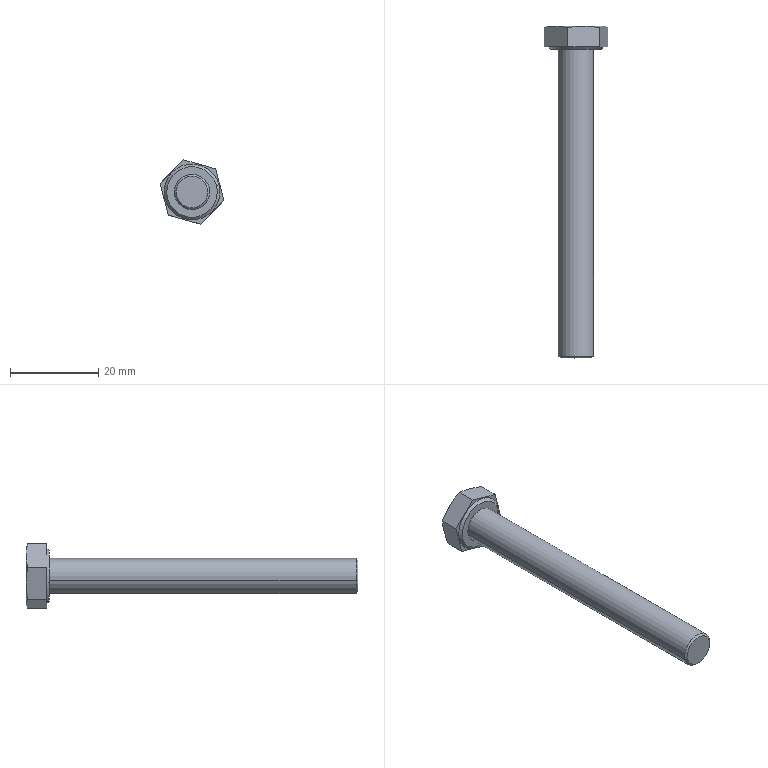Part | STEP file | 2026.6.15-Main Assembly图.sldasm-Part-12 | 1 solid | 22 faces | box 14.453 x 75.3 x 14.544 mm | volume 4272 mm3 | cone 10 | plane 10 | cylinder 2 | commonest cylinder face diameters 8 x2
STEP:
#1=CARTESIAN_POINT('',(-848.14,570.541,3100.088));
#2=VERTEX_POINT('',#1);
#3=CARTESIAN_POINT('',(-841.164,570.541,3101.869));
#4=VERTEX_POINT('',#3);
#5=CARTESIAN_POINT('',(-844.652,570.541,3100.979));
#6=DIRECTION('',(0.,-1.,0.));
#7=DIRECTION('',(-0.9689,0.,-0.2474));
#8=AXIS2_PLACEMENT_3D('',#5,#6,#7);
#9=CIRCLE('',#8,3.6);
#10=EDGE_CURVE('',#2,#4,#9,.T.);
#11=ORIENTED_EDGE('',*,*,#10,.F.);
#12=CARTESIAN_POINT('',(-848.527,570.941,3099.989));
#13=VERTEX_POINT('',#12);
#14=CARTESIAN_POINT('',(-848.14,570.541,3100.088));
#15=DIRECTION('',(-0.6851,0.7071,-0.1749));
#16=VECTOR('',#15,1000.);
#17=LINE('',#14,#16);
#18=EDGE_CURVE('',#2,#13,#17,.T.);
#19=ORIENTED_EDGE('',*,*,#18,.T.);
#20=CARTESIAN_POINT('',(-840.776,570.941,3101.968));
#21=VERTEX_POINT('',#20);
#22=CARTESIAN_POINT('',(-844.652,570.941,3100.979));
#23=DIRECTION('',(0.,1.,0.));
#24=DIRECTION('',(-0.9689,0.,-0.2474));
#25=AXIS2_PLACEMENT_3D('',#22,#23,#24);
#26=CIRCLE('',#25,4.);
#27=EDGE_CURVE('',#21,#13,#26,.T.);
#28=ORIENTED_EDGE('',*,*,#27,.F.);
#29=CARTESIAN_POINT('',(-841.164,570.541,3101.869));
#30=DIRECTION('',(0.6851,0.7071,0.1749));
#31=VECTOR('',#30,1000.);
#32=LINE('',#29,#31);
#33=EDGE_CURVE('',#4,#21,#32,.T.);
#34=ORIENTED_EDGE('',*,*,#33,.F.);
#35=EDGE_LOOP('',(#11,#19,#28,#34));
#36=FACE_OUTER_BOUND('',#35,.T.);
#37=CARTESIAN_POINT('',(-844.652,570.541,3100.979));
#38=DIRECTION('',(0.,1.,0.));
#39=DIRECTION('',(-0.9689,0.,-0.2474));
#40=AXIS2_PLACEMENT_3D('',#37,#38,#39);
#41=CONICAL_SURFACE('',#40,3.6,0.7854);
#42=ADVANCED_FACE('',(#36),#41,.T.);
#43=ORIENTED_EDGE('',*,*,#27,.T.);
#44=CARTESIAN_POINT('',(-848.527,640.541,3099.989));
#45=VERTEX_POINT('',#44);
#46=CARTESIAN_POINT('',(-848.527,570.541,3099.989));
#47=DIRECTION('',(0.,1.,0.));
#48=VECTOR('',#47,1000.);
#49=LINE('',#46,#48);
#50=EDGE_CURVE('',#13,#45,#49,.T.);
#51=ORIENTED_EDGE('',*,*,#50,.T.);
#52=CARTESIAN_POINT('',(-840.776,640.541,3101.968));
#53=VERTEX_POINT('',#52);
#54=CARTESIAN_POINT('',(-844.652,640.541,3100.979));
#55=DIRECTION('',(0.,-1.,0.));
#56=DIRECTION('',(0.9689,0.,0.2474));
#57=AXIS2_PLACEMENT_3D('',#54,#55,#56);
#58=CIRCLE('',#57,4.);
#59=EDGE_CURVE('',#45,#53,#58,.T.);
#60=ORIENTED_EDGE('',*,*,#59,.T.);
#61=CARTESIAN_POINT('',(-840.776,570.541,3101.968));
#62=DIRECTION('',(0.,1.,0.));
#63=VECTOR('',#62,1000.);
#64=LINE('',#61,#63);
#65=EDGE_CURVE('',#21,#53,#64,.T.);
#66=ORIENTED_EDGE('',*,*,#65,.F.);
#67=EDGE_LOOP('',(#43,#51,#60,#66));
#68=FACE_OUTER_BOUND('',#67,.T.);
#69=CARTESIAN_POINT('',(-844.652,570.541,3100.979));
#70=DIRECTION('',(0.,1.,0.));
#71=DIRECTION('',(-0.9689,0.,-0.2474));
#72=AXIS2_PLACEMENT_3D('',#69,#70,#71);
#73=CYLINDRICAL_SURFACE('',#72,4.);
#74=ADVANCED_FACE('',(#68),#73,.T.);
#75=CARTESIAN_POINT('',(-839.095,640.541,3102.398));
#76=VERTEX_POINT('',#75);
#77=CARTESIAN_POINT('',(-850.209,640.541,3099.56));
#78=VERTEX_POINT('',#77);
#79=CARTESIAN_POINT('',(-844.652,640.541,3100.979));
#80=DIRECTION('',(0.,1.,0.));
#81=DIRECTION('',(0.9689,0.,0.2474));
#82=AXIS2_PLACEMENT_3D('',#79,#80,#81);
#83=CIRCLE('',#82,5.735);
#84=EDGE_CURVE('',#76,#78,#83,.T.);
#85=ORIENTED_EDGE('',*,*,#84,.T.);
#86=CARTESIAN_POINT('',(-850.79,641.141,3099.412));
#87=VERTEX_POINT('',#86);
#88=CARTESIAN_POINT('',(-850.79,641.141,3099.412));
#89=DIRECTION('',(-0.6851,0.7071,-0.1749));
#90=VECTOR('',#89,1000.);
#91=LINE('',#88,#90);
#92=EDGE_CURVE('',#78,#87,#91,.T.);
#93=ORIENTED_EDGE('',*,*,#92,.T.);
#94=CARTESIAN_POINT('',(-838.514,641.141,3102.546));
#95=VERTEX_POINT('',#94);
#96=CARTESIAN_POINT('',(-844.652,641.141,3100.979));
#97=DIRECTION('',(0.,1.,0.));
#98=DIRECTION('',(0.9689,0.,0.2474));
#99=AXIS2_PLACEMENT_3D('',#96,#97,#98);
#100=CIRCLE('',#99,6.335);
#101=EDGE_CURVE('',#95,#87,#100,.T.);
#102=ORIENTED_EDGE('',*,*,#101,.F.);
#103=CARTESIAN_POINT('',(-838.514,641.141,3102.546));
#104=DIRECTION('',(0.6851,0.7071,0.1749));
#105=VECTOR('',#104,1000.);
#106=LINE('',#103,#105);
#107=EDGE_CURVE('',#76,#95,#106,.T.);
#108=ORIENTED_EDGE('',*,*,#107,.F.);
#109=EDGE_LOOP('',(#85,#93,#102,#108));
#110=FACE_OUTER_BOUND('',#109,.T.);
#111=CARTESIAN_POINT('',(-844.652,641.141,3100.979));
#112=DIRECTION('',(0.,1.,0.));
#113=DIRECTION('',(-0.9689,0.,-0.2474));
#114=AXIS2_PLACEMENT_3D('',#111,#112,#113);
#115=CONICAL_SURFACE('',#114,6.335,0.7854);
#116=ADVANCED_FACE('',(#110),#115,.T.);
#117=ORIENTED_EDGE('',*,*,#84,.F.);
#118=CARTESIAN_POINT('',(-844.652,640.541,3100.979));
#119=DIRECTION('',(0.,1.,0.));
#120=DIRECTION('',(0.9689,0.,0.2474));
#121=AXIS2_PLACEMENT_3D('',#118,#119,#120);
#122=CIRCLE('',#121,5.735);
#123=EDGE_CURVE('',#78,#76,#122,.T.);
#124=ORIENTED_EDGE('',*,*,#123,.F.);
#125=EDGE_LOOP('',(#117,#124));
#126=FACE_OUTER_BOUND('',#125,.T.);
#127=CARTESIAN_POINT('',(-844.652,640.541,3100.979));
#128=DIRECTION('',(0.,-1.,0.));
#129=DIRECTION('',(0.9689,0.,0.2474));
#130=AXIS2_PLACEMENT_3D('',#127,#128,#129);
#131=CIRCLE('',#130,4.);
#132=EDGE_CURVE('',#53,#45,#131,.T.);
#133=ORIENTED_EDGE('',*,*,#132,.F.);
#134=ORIENTED_EDGE('',*,*,#59,.F.);
#135=EDGE_LOOP('',(#133,#134));
#136=FACE_BOUND('',#135,.T.);
#137=CARTESIAN_POINT('',(-832.056,640.541,3104.195));
#138=DIRECTION('',(0.,1.,0.));
#139=DIRECTION('',(-0.9689,0.,-0.2474));
#140=AXIS2_PLACEMENT_3D('',#137,#138,#139);
#141=PLANE('',#140);
#142=ADVANCED_FACE('',(#126,#136),#141,.F.);
#143=CARTESIAN_POINT('',(-846.509,645.475,3108.251));
#144=VERTEX_POINT('',#143);
#145=CARTESIAN_POINT('',(-842.895,645.841,3107.237));
#146=VERTEX_POINT('',#145);
#147=CARTESIAN_POINT('',(-846.509,645.475,3108.251));
#148=CARTESIAN_POINT('',(-845.314,645.701,3107.916));
#149=CARTESIAN_POINT('',(-844.111,645.841,3107.578));
#150=CARTESIAN_POINT('',(-842.895,645.841,3107.237));
#151=B_SPLINE_CURVE_WITH_KNOTS('',3,(#147,#148,#149,#150),.UNSPECIFIED.,.F.,.F.,(4,4),(0.,0.003771),.UNSPECIFIED.);
#152=EDGE_CURVE('',#144,#146,#151,.T.);
#153=ORIENTED_EDGE('',*,*,#152,.F.);
#154=CARTESIAN_POINT('',(-846.509,641.141,3108.251));
#155=VERTEX_POINT('',#154);
#156=CARTESIAN_POINT('',(-846.509,640.541,3108.251));
#157=DIRECTION('',(0.,1.,0.));
#158=VECTOR('',#157,1000.);
#159=LINE('',#156,#158);
#160=EDGE_CURVE('',#155,#144,#159,.T.);
#161=ORIENTED_EDGE('',*,*,#160,.F.);
#162=CARTESIAN_POINT('',(-839.282,641.141,3106.223));
#163=VERTEX_POINT('',#162);
#164=CARTESIAN_POINT('',(-839.282,641.141,3106.223));
#165=DIRECTION('',(-0.9628,0.,0.2702));
#166=VECTOR('',#165,1000.);
#167=LINE('',#164,#166);
#168=EDGE_CURVE('',#163,#155,#167,.T.);
#169=ORIENTED_EDGE('',*,*,#168,.F.);
#170=CARTESIAN_POINT('',(-839.282,645.475,3106.223));
#171=VERTEX_POINT('',#170);
#172=CARTESIAN_POINT('',(-839.282,640.541,3106.223));
#173=DIRECTION('',(0.,1.,0.));
#174=VECTOR('',#173,1000.);
#175=LINE('',#172,#174);
#176=EDGE_CURVE('',#163,#171,#175,.T.);
#177=ORIENTED_EDGE('',*,*,#176,.T.);
#178=CARTESIAN_POINT('',(-842.895,645.841,3107.237));
#179=CARTESIAN_POINT('',(-841.68,645.841,3106.896));
#180=CARTESIAN_POINT('',(-840.477,645.701,3106.558));
#181=CARTESIAN_POINT('',(-839.282,645.475,3106.223));
#182=B_SPLINE_CURVE_WITH_KNOTS('',3,(#178,#179,#180,#181),.UNSPECIFIED.,.F.,.F.,(4,4),(0.,0.003771),.UNSPECIFIED.);
#183=EDGE_CURVE('',#146,#171,#182,.T.);
#184=ORIENTED_EDGE('',*,*,#183,.F.);
#185=EDGE_LOOP('',(#153,#161,#169,#177,#184));
#186=FACE_OUTER_BOUND('',#185,.T.);
#187=CARTESIAN_POINT('',(-839.282,640.541,3106.223));
#188=DIRECTION('',(-0.2702,0.,-0.9628));
#189=DIRECTION('',(0.,-1.,0.));
#190=AXIS2_PLACEMENT_3D('',#187,#188,#189);
#191=PLANE('',#190);
#192=ADVANCED_FACE('',(#186),#191,.F.);
#193=CARTESIAN_POINT('',(-851.878,645.475,3103.007));
#194=VERTEX_POINT('',#193);
#195=CARTESIAN_POINT('',(-849.193,645.841,3105.629));
#196=VERTEX_POINT('',#195);
#197=CARTESIAN_POINT('',(-851.878,645.475,3103.007));
#198=CARTESIAN_POINT('',(-850.991,645.701,3103.874));
#199=CARTESIAN_POINT('',(-850.097,645.841,3104.747));
#200=CARTESIAN_POINT('',(-849.193,645.841,3105.629));
#201=B_SPLINE_CURVE_WITH_KNOTS('',3,(#197,#198,#199,#200),.UNSPECIFIED.,.F.,.F.,(4,4),(0.,0.003771),.UNSPECIFIED.);
#202=EDGE_CURVE('',#194,#196,#201,.T.);
#203=ORIENTED_EDGE('',*,*,#202,.F.);
#204=CARTESIAN_POINT('',(-851.878,641.141,3103.007));
#205=VERTEX_POINT('',#204);
#206=CARTESIAN_POINT('',(-851.878,640.541,3103.007));
#207=DIRECTION('',(0.,1.,0.));
#208=VECTOR('',#207,1000.);
#209=LINE('',#206,#208);
#210=EDGE_CURVE('',#205,#194,#209,.T.);
#211=ORIENTED_EDGE('',*,*,#210,.F.);
#212=CARTESIAN_POINT('',(-846.509,641.141,3108.251));
#213=DIRECTION('',(-0.7154,0.,-0.6987));
#214=VECTOR('',#213,1000.);
#215=LINE('',#212,#214);
#216=EDGE_CURVE('',#155,#205,#215,.T.);
#217=ORIENTED_EDGE('',*,*,#216,.F.);
#218=ORIENTED_EDGE('',*,*,#160,.T.);
#219=CARTESIAN_POINT('',(-849.193,645.841,3105.629));
#220=CARTESIAN_POINT('',(-848.29,645.841,3106.511));
#221=CARTESIAN_POINT('',(-847.396,645.701,3107.384));
#222=CARTESIAN_POINT('',(-846.509,645.475,3108.251));
#223=B_SPLINE_CURVE_WITH_KNOTS('',3,(#219,#220,#221,#222),.UNSPECIFIED.,.F.,.F.,(4,4),(0.,0.003771),.UNSPECIFIED.);
#224=EDGE_CURVE('',#196,#144,#223,.T.);
#225=ORIENTED_EDGE('',*,*,#224,.F.);
#226=EDGE_LOOP('',(#203,#211,#217,#218,#225));
#227=FACE_OUTER_BOUND('',#226,.T.);
#228=CARTESIAN_POINT('',(-846.509,640.541,3108.251));
#229=DIRECTION('',(0.6987,0.,-0.7154));
#230=DIRECTION('',(0.,1.,0.));
#231=AXIS2_PLACEMENT_3D('',#228,#229,#230);
#232=PLANE('',#231);
#233=ADVANCED_FACE('',(#227),#232,.F.);
#234=CARTESIAN_POINT('',(-850.021,645.475,3095.735));
#235=VERTEX_POINT('',#234);
#236=CARTESIAN_POINT('',(-850.95,645.841,3099.371));
#237=VERTEX_POINT('',#236);
#238=CARTESIAN_POINT('',(-850.021,645.475,3095.735));
#239=CARTESIAN_POINT('',(-850.328,645.701,3096.937));
#240=CARTESIAN_POINT('',(-850.637,645.841,3098.147));
#241=CARTESIAN_POINT('',(-850.95,645.841,3099.371));
#242=B_SPLINE_CURVE_WITH_KNOTS('',3,(#238,#239,#240,#241),.UNSPECIFIED.,.F.,.F.,(4,4),(0.,0.003771),.UNSPECIFIED.);
#243=EDGE_CURVE('',#235,#237,#242,.T.);
#244=ORIENTED_EDGE('',*,*,#243,.F.);
#245=CARTESIAN_POINT('',(-850.021,641.141,3095.735));
#246=VERTEX_POINT('',#245);
#247=CARTESIAN_POINT('',(-850.021,640.541,3095.735));
#248=DIRECTION('',(0.,1.,0.));
#249=VECTOR('',#248,1000.);
#250=LINE('',#247,#249);
#251=EDGE_CURVE('',#246,#235,#250,.T.);
#252=ORIENTED_EDGE('',*,*,#251,.F.);
#253=CARTESIAN_POINT('',(-851.878,641.141,3103.007));
#254=DIRECTION('',(0.2474,0.,-0.9689));
#255=VECTOR('',#254,1000.);
#256=LINE('',#253,#255);
#257=EDGE_CURVE('',#205,#246,#256,.T.);
#258=ORIENTED_EDGE('',*,*,#257,.F.);
#259=ORIENTED_EDGE('',*,*,#210,.T.);
#260=CARTESIAN_POINT('',(-850.95,645.841,3099.371));
#261=CARTESIAN_POINT('',(-851.262,645.841,3100.594));
#262=CARTESIAN_POINT('',(-851.571,645.701,3101.805));
#263=CARTESIAN_POINT('',(-851.878,645.475,3103.007));
#264=B_SPLINE_CURVE_WITH_KNOTS('',3,(#260,#261,#262,#263),.UNSPECIFIED.,.F.,.F.,(4,4),(0.,0.003771),.UNSPECIFIED.);
#265=EDGE_CURVE('',#237,#194,#264,.T.);
#266=ORIENTED_EDGE('',*,*,#265,.F.);
#267=EDGE_LOOP('',(#244,#252,#258,#259,#266));
#268=FACE_OUTER_BOUND('',#267,.T.);
#269=CARTESIAN_POINT('',(-851.878,640.541,3103.007));
#270=DIRECTION('',(0.9689,0.,0.2474));
#271=DIRECTION('',(0.2474,0.,-0.9689));
#272=AXIS2_PLACEMENT_3D('',#269,#270,#271);
#273=PLANE('',#272);
#274=ADVANCED_FACE('',(#268),#273,.F.);
#275=CARTESIAN_POINT('',(-842.795,645.475,3093.707));
#276=VERTEX_POINT('',#275);
#277=CARTESIAN_POINT('',(-846.408,645.841,3094.721));
#278=VERTEX_POINT('',#277);
#279=CARTESIAN_POINT('',(-842.795,645.475,3093.707));
#280=CARTESIAN_POINT('',(-843.99,645.701,3094.042));
#281=CARTESIAN_POINT('',(-845.192,645.841,3094.379));
#282=CARTESIAN_POINT('',(-846.408,645.841,3094.721));
#283=B_SPLINE_CURVE_WITH_KNOTS('',3,(#279,#280,#281,#282),.UNSPECIFIED.,.F.,.F.,(4,4),(0.,0.003771),.UNSPECIFIED.);
#284=EDGE_CURVE('',#276,#278,#283,.T.);
#285=ORIENTED_EDGE('',*,*,#284,.F.);
#286=CARTESIAN_POINT('',(-842.795,641.141,3093.707));
#287=VERTEX_POINT('',#286);
#288=CARTESIAN_POINT('',(-842.795,640.541,3093.707));
#289=DIRECTION('',(0.,1.,0.));
#290=VECTOR('',#289,1000.);
#291=LINE('',#288,#290);
#292=EDGE_CURVE('',#287,#276,#291,.T.);
#293=ORIENTED_EDGE('',*,*,#292,.F.);
#294=CARTESIAN_POINT('',(-850.021,641.141,3095.735));
#295=DIRECTION('',(0.9628,0.,-0.2702));
#296=VECTOR('',#295,1000.);
#297=LINE('',#294,#296);
#298=EDGE_CURVE('',#246,#287,#297,.T.);
#299=ORIENTED_EDGE('',*,*,#298,.F.);
#300=ORIENTED_EDGE('',*,*,#251,.T.);
#301=CARTESIAN_POINT('',(-846.408,645.841,3094.721));
#302=CARTESIAN_POINT('',(-847.624,645.841,3095.062));
#303=CARTESIAN_POINT('',(-848.827,645.701,3095.399));
#304=CARTESIAN_POINT('',(-850.021,645.475,3095.735));
#305=B_SPLINE_CURVE_WITH_KNOTS('',3,(#301,#302,#303,#304),.UNSPECIFIED.,.F.,.F.,(4,4),(0.,0.003771),.UNSPECIFIED.);
#306=EDGE_CURVE('',#278,#235,#305,.T.);
#307=ORIENTED_EDGE('',*,*,#306,.F.);
#308=EDGE_LOOP('',(#285,#293,#299,#300,#307));
#309=FACE_OUTER_BOUND('',#308,.T.);
#310=CARTESIAN_POINT('',(-850.021,640.541,3095.735));
#311=DIRECTION('',(0.2702,0.,0.9628));
#312=DIRECTION('',(0.,-1.,0.));
#313=AXIS2_PLACEMENT_3D('',#310,#311,#312);
#314=PLANE('',#313);
#315=ADVANCED_FACE('',(#309),#314,.F.);
#316=CARTESIAN_POINT('',(-837.425,645.475,3098.951));
#317=VERTEX_POINT('',#316);
#318=CARTESIAN_POINT('',(-840.11,645.841,3096.329));
#319=VERTEX_POINT('',#318);
#320=CARTESIAN_POINT('',(-837.425,645.475,3098.951));
#321=CARTESIAN_POINT('',(-838.313,645.701,3098.084));
#322=CARTESIAN_POINT('',(-839.207,645.841,3097.211));
#323=CARTESIAN_POINT('',(-840.11,645.841,3096.329));
#324=B_SPLINE_CURVE_WITH_KNOTS('',3,(#320,#321,#322,#323),.UNSPECIFIED.,.F.,.F.,(4,4),(0.,0.003771),.UNSPECIFIED.);
#325=EDGE_CURVE('',#317,#319,#324,.T.);
#326=ORIENTED_EDGE('',*,*,#325,.F.);
#327=CARTESIAN_POINT('',(-837.425,641.141,3098.951));
#328=VERTEX_POINT('',#327);
#329=CARTESIAN_POINT('',(-837.425,640.541,3098.951));
#330=DIRECTION('',(0.,1.,0.));
#331=VECTOR('',#330,1000.);
#332=LINE('',#329,#331);
#333=EDGE_CURVE('',#328,#317,#332,.T.);
#334=ORIENTED_EDGE('',*,*,#333,.F.);
#335=CARTESIAN_POINT('',(-842.795,641.141,3093.707));
#336=DIRECTION('',(0.7154,0.,0.6987));
#337=VECTOR('',#336,1000.);
#338=LINE('',#335,#337);
#339=EDGE_CURVE('',#287,#328,#338,.T.);
#340=ORIENTED_EDGE('',*,*,#339,.F.);
#341=ORIENTED_EDGE('',*,*,#292,.T.);
#342=CARTESIAN_POINT('',(-840.11,645.841,3096.329));
#343=CARTESIAN_POINT('',(-841.014,645.841,3095.446));
#344=CARTESIAN_POINT('',(-841.907,645.701,3094.574));
#345=CARTESIAN_POINT('',(-842.795,645.475,3093.707));
#346=B_SPLINE_CURVE_WITH_KNOTS('',3,(#342,#343,#344,#345),.UNSPECIFIED.,.F.,.F.,(4,4),(0.,0.003771),.UNSPECIFIED.);
#347=EDGE_CURVE('',#319,#276,#346,.T.);
#348=ORIENTED_EDGE('',*,*,#347,.F.);
#349=EDGE_LOOP('',(#326,#334,#340,#341,#348));
#350=FACE_OUTER_BOUND('',#349,.T.);
#351=CARTESIAN_POINT('',(-842.795,640.541,3093.707));
#352=DIRECTION('',(-0.6987,0.,0.7154));
#353=DIRECTION('',(0.7154,0.,0.6987));
#354=AXIS2_PLACEMENT_3D('',#351,#352,#353);
#355=PLANE('',#354);
#356=ADVANCED_FACE('',(#350),#355,.F.);
#357=CARTESIAN_POINT('',(-838.354,645.841,3102.587));
#358=VERTEX_POINT('',#357);
#359=CARTESIAN_POINT('',(-839.282,645.475,3106.223));
#360=CARTESIAN_POINT('',(-838.975,645.701,3105.021));
#361=CARTESIAN_POINT('',(-838.666,645.841,3103.811));
#362=CARTESIAN_POINT('',(-838.354,645.841,3102.587));
#363=B_SPLINE_CURVE_WITH_KNOTS('',3,(#359,#360,#361,#362),.UNSPECIFIED.,.F.,.F.,(4,4),(0.,0.003771),.UNSPECIFIED.);
#364=EDGE_CURVE('',#171,#358,#363,.T.);
#365=ORIENTED_EDGE('',*,*,#364,.F.);
#366=ORIENTED_EDGE('',*,*,#176,.F.);
#367=CARTESIAN_POINT('',(-837.425,641.141,3098.951));
#368=DIRECTION('',(-0.2474,0.,0.9689));
#369=VECTOR('',#368,1000.);
#370=LINE('',#367,#369);
#371=EDGE_CURVE('',#328,#163,#370,.T.);
#372=ORIENTED_EDGE('',*,*,#371,.F.);
#373=ORIENTED_EDGE('',*,*,#333,.T.);
#374=CARTESIAN_POINT('',(-838.354,645.841,3102.587));
#375=CARTESIAN_POINT('',(-838.041,645.841,3101.363));
#376=CARTESIAN_POINT('',(-837.732,645.701,3100.153));
#377=CARTESIAN_POINT('',(-837.425,645.475,3098.951));
#378=B_SPLINE_CURVE_WITH_KNOTS('',3,(#374,#375,#376,#377),.UNSPECIFIED.,.F.,.F.,(4,4),(0.,0.003771),.UNSPECIFIED.);
#379=EDGE_CURVE('',#358,#317,#378,.T.);
#380=ORIENTED_EDGE('',*,*,#379,.F.);
#381=EDGE_LOOP('',(#365,#366,#372,#373,#380));
#382=FACE_OUTER_BOUND('',#381,.T.);
#383=CARTESIAN_POINT('',(-837.425,640.541,3098.951));
#384=DIRECTION('',(-0.9689,0.,-0.2474));
#385=DIRECTION('',(0.2474,0.,-0.9689));
#386=AXIS2_PLACEMENT_3D('',#383,#384,#385);
#387=PLANE('',#386);
#388=ADVANCED_FACE('',(#382),#387,.F.);
#389=ORIENTED_EDGE('',*,*,#168,.T.);
#390=ORIENTED_EDGE('',*,*,#216,.T.);
#391=ORIENTED_EDGE('',*,*,#257,.T.);
#392=ORIENTED_EDGE('',*,*,#298,.T.);
#393=ORIENTED_EDGE('',*,*,#339,.T.);
#394=ORIENTED_EDGE('',*,*,#371,.T.);
#395=EDGE_LOOP('',(#389,#390,#391,#392,#393,#394));
#396=FACE_OUTER_BOUND('',#395,.T.);
#397=ORIENTED_EDGE('',*,*,#101,.T.);
#398=CARTESIAN_POINT('',(-844.652,641.141,3100.979));
#399=DIRECTION('',(0.,1.,0.));
#400=DIRECTION('',(0.9689,0.,0.2474));
#401=AXIS2_PLACEMENT_3D('',#398,#399,#400);
#402=CIRCLE('',#401,6.335);
#403=EDGE_CURVE('',#87,#95,#402,.T.);
#404=ORIENTED_EDGE('',*,*,#403,.T.);
#405=EDGE_LOOP('',(#397,#404));
#406=FACE_BOUND('',#405,.T.);
#407=CARTESIAN_POINT('',(-843.085,641.141,3094.841));
#408=DIRECTION('',(0.,-1.,0.));
#409=DIRECTION('',(-0.2474,0.,0.9689));
#410=AXIS2_PLACEMENT_3D('',#407,#408,#409);
#411=PLANE('',#410);
#412=ADVANCED_FACE('',(#396,#406),#411,.T.);
#413=ORIENTED_EDGE('',*,*,#92,.F.);
#414=ORIENTED_EDGE('',*,*,#123,.T.);
#415=ORIENTED_EDGE('',*,*,#107,.T.);
#416=ORIENTED_EDGE('',*,*,#403,.F.);
#417=EDGE_LOOP('',(#413,#414,#415,#416));
#418=FACE_OUTER_BOUND('',#417,.T.);
#419=CARTESIAN_POINT('',(-844.652,641.141,3100.979));
#420=DIRECTION('',(0.,1.,0.));
#421=DIRECTION('',(-0.9689,0.,-0.2474));
#422=AXIS2_PLACEMENT_3D('',#419,#420,#421);
#423=CONICAL_SURFACE('',#422,6.335,0.7854);
#424=ADVANCED_FACE('',(#418),#423,.T.);
#425=ORIENTED_EDGE('',*,*,#183,.T.);
#426=ORIENTED_EDGE('',*,*,#364,.T.);
#427=CARTESIAN_POINT('',(-844.652,645.841,3100.979));
#428=DIRECTION('',(0.,1.,0.));
#429=DIRECTION('',(0.9689,0.,0.2474));
#430=AXIS2_PLACEMENT_3D('',#427,#428,#429);
#431=CIRCLE('',#430,6.5);
#432=EDGE_CURVE('',#146,#358,#431,.T.);
#433=ORIENTED_EDGE('',*,*,#432,.F.);
#434=EDGE_LOOP('',(#425,#426,#433));
#435=FACE_OUTER_BOUND('',#434,.T.);
#436=CARTESIAN_POINT('',(-844.652,645.841,3100.979));
#437=DIRECTION('',(0.,-1.,0.));
#438=DIRECTION('',(0.9689,0.,0.2474));
#439=AXIS2_PLACEMENT_3D('',#436,#437,#438);
#440=CONICAL_SURFACE('',#439,6.5,1.222);
#441=ADVANCED_FACE('',(#435),#440,.T.);
#442=ORIENTED_EDGE('',*,*,#224,.T.);
#443=ORIENTED_EDGE('',*,*,#152,.T.);
#444=CARTESIAN_POINT('',(-844.652,645.841,3100.979));
#445=DIRECTION('',(0.,1.,0.));
#446=DIRECTION('',(0.9689,0.,0.2474));
#447=AXIS2_PLACEMENT_3D('',#444,#445,#446);
#448=CIRCLE('',#447,6.5);
#449=EDGE_CURVE('',#196,#146,#448,.T.);
#450=ORIENTED_EDGE('',*,*,#449,.F.);
#451=EDGE_LOOP('',(#442,#443,#450));
#452=FACE_OUTER_BOUND('',#451,.T.);
#453=CARTESIAN_POINT('',(-844.652,645.841,3100.979));
#454=DIRECTION('',(0.,-1.,0.));
#455=DIRECTION('',(0.9689,0.,0.2474));
#456=AXIS2_PLACEMENT_3D('',#453,#454,#455);
#457=CONICAL_SURFACE('',#456,6.5,1.222);
#458=ADVANCED_FACE('',(#452),#457,.T.);
#459=ORIENTED_EDGE('',*,*,#265,.T.);
#460=ORIENTED_EDGE('',*,*,#202,.T.);
#461=CARTESIAN_POINT('',(-844.652,645.841,3100.979));
#462=DIRECTION('',(0.,1.,0.));
#463=DIRECTION('',(0.9689,0.,0.2474));
#464=AXIS2_PLACEMENT_3D('',#461,#462,#463);
#465=CIRCLE('',#464,6.5);
#466=EDGE_CURVE('',#237,#196,#465,.T.);
#467=ORIENTED_EDGE('',*,*,#466,.F.);
#468=EDGE_LOOP('',(#459,#460,#467));
#469=FACE_OUTER_BOUND('',#468,.T.);
#470=CARTESIAN_POINT('',(-844.652,645.841,3100.979));
#471=DIRECTION('',(0.,-1.,0.));
#472=DIRECTION('',(0.9689,0.,0.2474));
#473=AXIS2_PLACEMENT_3D('',#470,#471,#472);
#474=CONICAL_SURFACE('',#473,6.5,1.222);
#475=ADVANCED_FACE('',(#469),#474,.T.);
#476=ORIENTED_EDGE('',*,*,#243,.T.);
#477=CARTESIAN_POINT('',(-844.652,645.841,3100.979));
#478=DIRECTION('',(0.,1.,0.));
#479=DIRECTION('',(0.9689,0.,0.2474));
#480=AXIS2_PLACEMENT_3D('',#477,#478,#479);
#481=CIRCLE('',#480,6.5);
#482=EDGE_CURVE('',#278,#237,#481,.T.);
#483=ORIENTED_EDGE('',*,*,#482,.F.);
#484=ORIENTED_EDGE('',*,*,#306,.T.);
#485=EDGE_LOOP('',(#476,#483,#484));
#486=FACE_OUTER_BOUND('',#485,.T.);
#487=CARTESIAN_POINT('',(-844.652,645.841,3100.979));
#488=DIRECTION('',(0.,-1.,0.));
#489=DIRECTION('',(0.9689,0.,0.2474));
#490=AXIS2_PLACEMENT_3D('',#487,#488,#489);
#491=CONICAL_SURFACE('',#490,6.5,1.222);
#492=ADVANCED_FACE('',(#486),#491,.T.);
#493=ORIENTED_EDGE('',*,*,#284,.T.);
#494=CARTESIAN_POINT('',(-844.652,645.841,3100.979));
#495=DIRECTION('',(0.,1.,0.));
#496=DIRECTION('',(0.9689,0.,0.2474));
#497=AXIS2_PLACEMENT_3D('',#494,#495,#496);
#498=CIRCLE('',#497,6.5);
#499=EDGE_CURVE('',#319,#278,#498,.T.);
#500=ORIENTED_EDGE('',*,*,#499,.F.);
#501=ORIENTED_EDGE('',*,*,#347,.T.);
#502=EDGE_LOOP('',(#493,#500,#501));
#503=FACE_OUTER_BOUND('',#502,.T.);
#504=CARTESIAN_POINT('',(-844.652,645.841,3100.979));
#505=DIRECTION('',(0.,-1.,0.));
#506=DIRECTION('',(0.9689,0.,0.2474));
#507=AXIS2_PLACEMENT_3D('',#504,#505,#506);
#508=CONICAL_SURFACE('',#507,6.5,1.222);
#509=ADVANCED_FACE('',(#503),#508,.T.);
#510=ORIENTED_EDGE('',*,*,#325,.T.);
#511=CARTESIAN_POINT('',(-844.652,645.841,3100.979));
#512=DIRECTION('',(0.,1.,0.));
#513=DIRECTION('',(0.9689,0.,0.2474));
#514=AXIS2_PLACEMENT_3D('',#511,#512,#513);
#515=CIRCLE('',#514,6.5);
#516=EDGE_CURVE('',#358,#319,#515,.T.);
#517=ORIENTED_EDGE('',*,*,#516,.F.);
#518=ORIENTED_EDGE('',*,*,#379,.T.);
#519=EDGE_LOOP('',(#510,#517,#518));
#520=FACE_OUTER_BOUND('',#519,.T.);
#521=CARTESIAN_POINT('',(-844.652,645.841,3100.979));
#522=DIRECTION('',(0.,-1.,0.));
#523=DIRECTION('',(0.9689,0.,0.2474));
#524=AXIS2_PLACEMENT_3D('',#521,#522,#523);
#525=CONICAL_SURFACE('',#524,6.5,1.222);
#526=ADVANCED_FACE('',(#520),#525,.T.);
#527=ORIENTED_EDGE('',*,*,#432,.T.);
#528=ORIENTED_EDGE('',*,*,#516,.T.);
#529=ORIENTED_EDGE('',*,*,#499,.T.);
#530=ORIENTED_EDGE('',*,*,#482,.T.);
#531=ORIENTED_EDGE('',*,*,#466,.T.);
#532=ORIENTED_EDGE('',*,*,#449,.T.);
#533=EDGE_LOOP('',(#527,#528,#529,#530,#531,#532));
#534=FACE_OUTER_BOUND('',#533,.T.);
#535=CARTESIAN_POINT('',(-832.056,645.841,3104.195));
#536=DIRECTION('',(0.,1.,0.));
#537=DIRECTION('',(-0.9689,0.,-0.2474));
#538=AXIS2_PLACEMENT_3D('',#535,#536,#537);
#539=PLANE('',#538);
#540=ADVANCED_FACE('',(#534),#539,.T.);
#541=ORIENTED_EDGE('',*,*,#50,.F.);
#542=CARTESIAN_POINT('',(-844.652,570.941,3100.979));
#543=DIRECTION('',(0.,1.,0.));
#544=DIRECTION('',(-0.9689,0.,-0.2474));
#545=AXIS2_PLACEMENT_3D('',#542,#543,#544);
#546=CIRCLE('',#545,4.);
#547=EDGE_CURVE('',#13,#21,#546,.T.);
#548=ORIENTED_EDGE('',*,*,#547,.T.);
#549=ORIENTED_EDGE('',*,*,#65,.T.);
#550=ORIENTED_EDGE('',*,*,#132,.T.);
#551=EDGE_LOOP('',(#541,#548,#549,#550));
#552=FACE_OUTER_BOUND('',#551,.T.);
#553=CARTESIAN_POINT('',(-844.652,570.541,3100.979));
#554=DIRECTION('',(0.,1.,0.));
#555=DIRECTION('',(-0.9689,0.,-0.2474));
#556=AXIS2_PLACEMENT_3D('',#553,#554,#555);
#557=CYLINDRICAL_SURFACE('',#556,4.);
#558=ADVANCED_FACE('',(#552),#557,.T.);
#559=CARTESIAN_POINT('',(-844.652,570.541,3100.979));
#560=DIRECTION('',(0.,-1.,0.));
#561=DIRECTION('',(-0.9689,0.,-0.2474));
#562=AXIS2_PLACEMENT_3D('',#559,#560,#561);
#563=CIRCLE('',#562,3.6);
#564=EDGE_CURVE('',#4,#2,#563,.T.);
#565=ORIENTED_EDGE('',*,*,#564,.T.);
#566=ORIENTED_EDGE('',*,*,#10,.T.);
#567=EDGE_LOOP('',(#565,#566));
#568=FACE_OUTER_BOUND('',#567,.T.);
#569=CARTESIAN_POINT('',(-844.652,570.541,3100.979));
#570=DIRECTION('',(0.,-1.,0.));
#571=DIRECTION('',(-0.2474,0.,0.9689));
#572=AXIS2_PLACEMENT_3D('',#569,#570,#571);
#573=PLANE('',#572);
#574=ADVANCED_FACE('',(#568),#573,.T.);
#575=ORIENTED_EDGE('',*,*,#18,.F.);
#576=ORIENTED_EDGE('',*,*,#564,.F.);
#577=ORIENTED_EDGE('',*,*,#33,.T.);
#578=ORIENTED_EDGE('',*,*,#547,.F.);
#579=EDGE_LOOP('',(#575,#576,#577,#578));
#580=FACE_OUTER_BOUND('',#579,.T.);
#581=CARTESIAN_POINT('',(-844.652,570.541,3100.979));
#582=DIRECTION('',(0.,1.,0.));
#583=DIRECTION('',(-0.9689,0.,-0.2474));
#584=AXIS2_PLACEMENT_3D('',#581,#582,#583);
#585=CONICAL_SURFACE('',#584,3.6,0.7854);
#586=ADVANCED_FACE('',(#580),#585,.T.);
#587=CLOSED_SHELL('',(#42,#74,#116,#142,#192,#233,#274,#315,#356,#388,#412,#424,#441,#458,#475,#492,#509,#526,#540,#558,#574,#586));
#588=MANIFOLD_SOLID_BREP('',#587);
#589=CARTESIAN_POINT('',(0.,0.,0.));
#590=DIRECTION('',(0.,0.,1.));
#591=DIRECTION('',(1.,0.,0.));
#592=AXIS2_PLACEMENT_3D('',#589,#590,#591);
#593=(LENGTH_UNIT()NAMED_UNIT(*)SI_UNIT(.MILLI.,.METRE.));
#594=UNCERTAINTY_MEASURE_WITH_UNIT(LENGTH_MEASURE(0.00001),#593,'','');
#595=(NAMED_UNIT(*)PLANE_ANGLE_UNIT()SI_UNIT($,.RADIAN.));
#596=(NAMED_UNIT(*)SI_UNIT($,.STERADIAN.)SOLID_ANGLE_UNIT());
#597=(GEOMETRIC_REPRESENTATION_CONTEXT(3)GLOBAL_UNCERTAINTY_ASSIGNED_CONTEXT((#594))GLOBAL_UNIT_ASSIGNED_CONTEXT((#593,#595,#596))REPRESENTATION_CONTEXT('',''));
#598=ADVANCED_BREP_SHAPE_REPRESENTATION('',(#588,#592),#597);